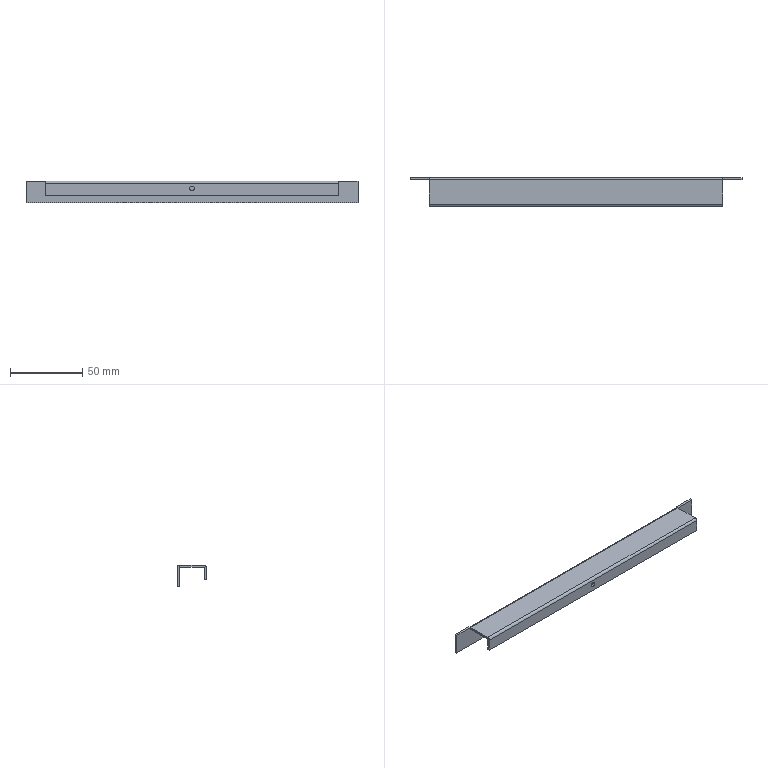Part | STEP file | HESS-408-70-15W-D-9-edge strip 1 | 1 solid | 24 faces | box 230 x 20 x 15 mm | volume 13161 mm3 | plane 18 | cylinder 6 | commonest cylinder face diameters 3.2 x4 0.2 x2